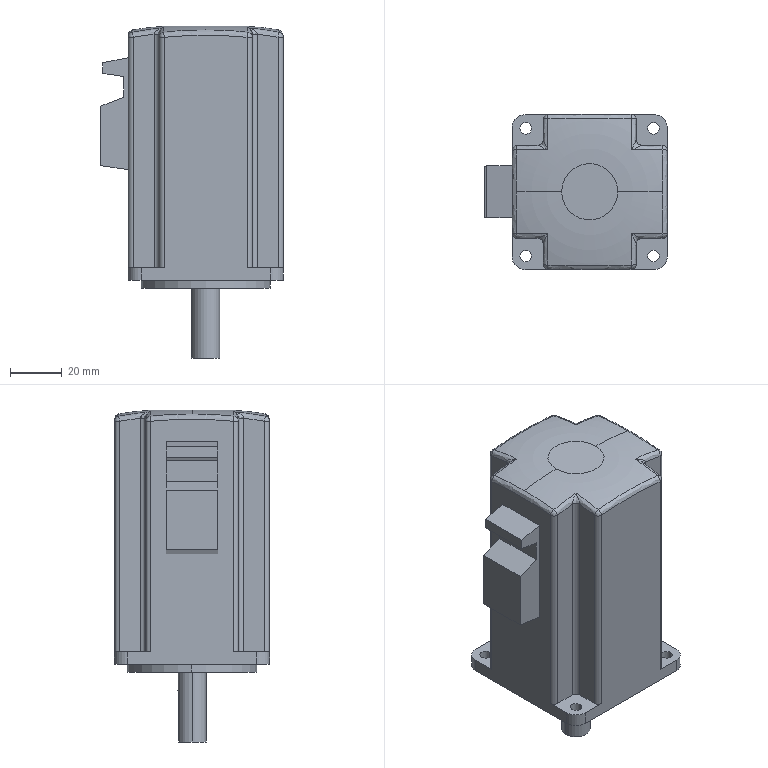Part | NX | features BREP 1 | 1 solid | 90 faces | box 70.588 x 60 x 128.5 mm | volume 308529 mm3 | plane 33 | cylinder 31 | spline 16 | sphere 8 | torus 2 | commonest cylinder face diameters 4 x13 4.5 x8 10 x4 11 x2 43.339 x2 50 x2